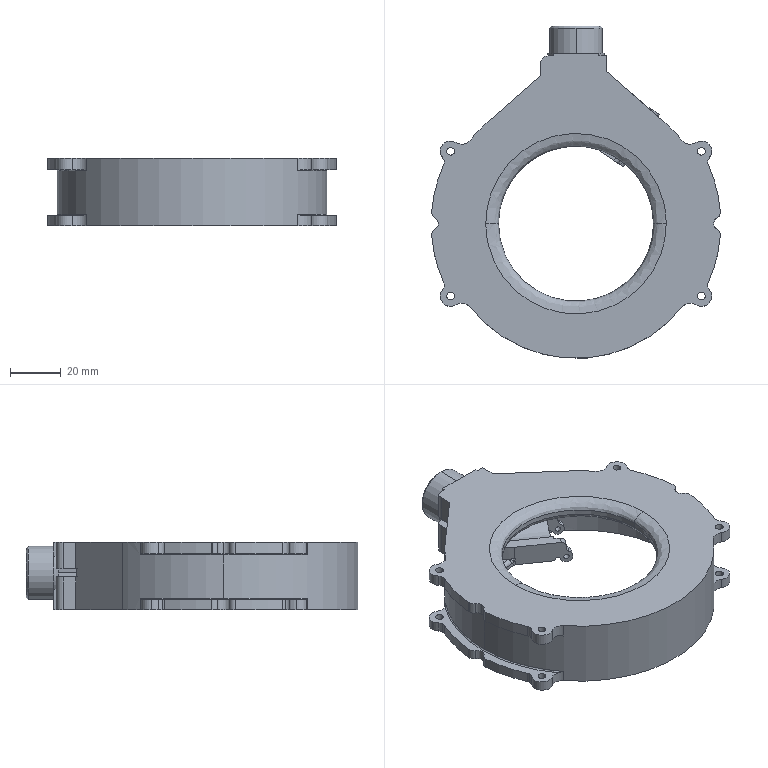Part | SolidWorks | features ICE 42, Fillet 29, Chamfer 4, Extrusion 1, RevCut 1, SweepCut 1 | 1 solid | 237 faces | box 113.626 x 130.8 x 26.5 mm | volume 67573 mm3 | cylinder 153 | plane 44 | torus 25 | spline 9 | sphere 4 | cone 2 | commonest cylinder face diameters 5 x40 2.1 x16 3.1 x16 8.1 x12 8.632 x8 114 x8